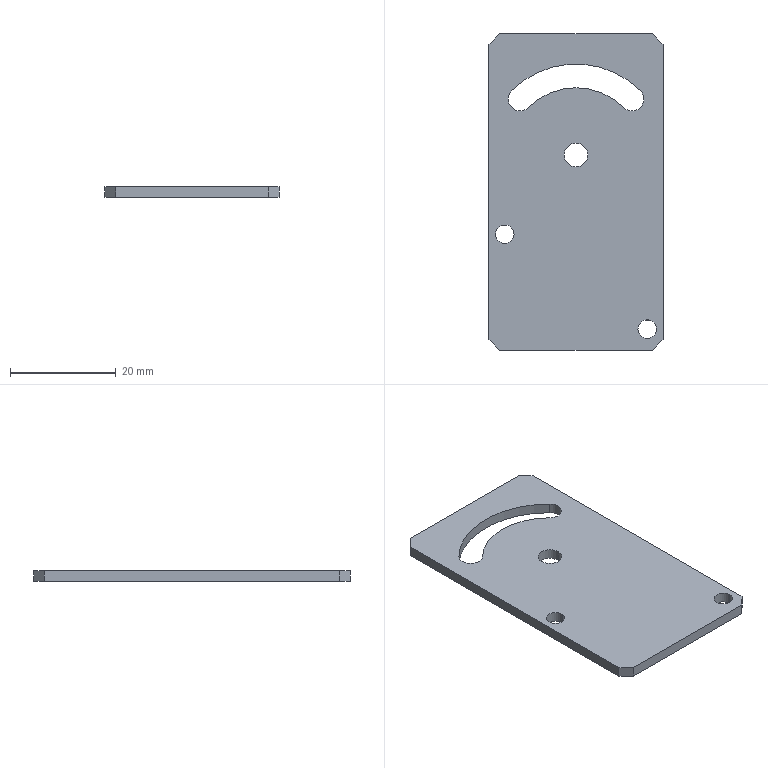Part | SolidWorks | features Chamfer 1, Extrusion 1 | 1 solid | 21 faces | box 33 x 60 x 2 mm | volume 3630 mm3 | cylinder 11 | plane 10 | commonest cylinder face diameters 4.5 x5 3.5 x4 25.5 x1 34.5 x1
STEP:
#1=CARTESIAN_POINT('',(-12.198,19.198,2.));
#2=VERTEX_POINT('',#1);
#3=CARTESIAN_POINT('',(-12.857,17.607,2.));
#4=VERTEX_POINT('',#3);
#5=CARTESIAN_POINT('',(-10.607,17.607,2.));
#6=DIRECTION('',(0.,0.,1.));
#7=DIRECTION('',(1.,0.,0.));
#8=AXIS2_PLACEMENT_3D('',#5,#6,#7);
#9=CIRCLE('',#8,2.25);
#10=EDGE_CURVE('',#2,#4,#9,.T.);
#11=ORIENTED_EDGE('',*,*,#10,.T.);
#12=CARTESIAN_POINT('',(-12.857,17.607,0.));
#13=VERTEX_POINT('',#12);
#14=CARTESIAN_POINT('',(-12.857,17.607,2.));
#15=DIRECTION('',(0.,0.,-1.));
#16=VECTOR('',#15,1000.);
#17=LINE('',#14,#16);
#18=EDGE_CURVE('',#4,#13,#17,.T.);
#19=ORIENTED_EDGE('',*,*,#18,.T.);
#20=CARTESIAN_POINT('',(-12.198,19.198,0.));
#21=VERTEX_POINT('',#20);
#22=CARTESIAN_POINT('',(-10.607,17.607,0.));
#23=DIRECTION('',(0.,0.,1.));
#24=DIRECTION('',(1.,0.,0.));
#25=AXIS2_PLACEMENT_3D('',#22,#23,#24);
#26=CIRCLE('',#25,2.25);
#27=EDGE_CURVE('',#21,#13,#26,.T.);
#28=ORIENTED_EDGE('',*,*,#27,.F.);
#29=CARTESIAN_POINT('',(-12.198,19.198,2.));
#30=DIRECTION('',(0.,0.,-1.));
#31=VECTOR('',#30,1000.);
#32=LINE('',#29,#31);
#33=EDGE_CURVE('',#2,#21,#32,.T.);
#34=ORIENTED_EDGE('',*,*,#33,.F.);
#35=EDGE_LOOP('',(#11,#19,#28,#34));
#36=FACE_OUTER_BOUND('',#35,.T.);
#37=CARTESIAN_POINT('',(-10.607,17.607,2.));
#38=DIRECTION('',(0.,0.,-1.));
#39=DIRECTION('',(-1.,0.,0.));
#40=AXIS2_PLACEMENT_3D('',#37,#38,#39);
#41=CYLINDRICAL_SURFACE('',#40,2.25);
#42=ADVANCED_FACE('',(#36),#41,.F.);
#43=CARTESIAN_POINT('',(-15.25,-8.,2.));
#44=VERTEX_POINT('',#43);
#45=CARTESIAN_POINT('',(-11.75,-8.,2.));
#46=VERTEX_POINT('',#45);
#47=CARTESIAN_POINT('',(-13.5,-8.,2.));
#48=DIRECTION('',(0.,0.,1.));
#49=DIRECTION('',(1.,0.,0.));
#50=AXIS2_PLACEMENT_3D('',#47,#48,#49);
#51=CIRCLE('',#50,1.75);
#52=EDGE_CURVE('',#44,#46,#51,.T.);
#53=ORIENTED_EDGE('',*,*,#52,.T.);
#54=CARTESIAN_POINT('',(-11.75,-8.,0.));
#55=VERTEX_POINT('',#54);
#56=CARTESIAN_POINT('',(-11.75,-8.,2.));
#57=DIRECTION('',(0.,0.,-1.));
#58=VECTOR('',#57,1000.);
#59=LINE('',#56,#58);
#60=EDGE_CURVE('',#46,#55,#59,.T.);
#61=ORIENTED_EDGE('',*,*,#60,.T.);
#62=CARTESIAN_POINT('',(-15.25,-8.,0.));
#63=VERTEX_POINT('',#62);
#64=CARTESIAN_POINT('',(-13.5,-8.,0.));
#65=DIRECTION('',(0.,0.,1.));
#66=DIRECTION('',(1.,0.,0.));
#67=AXIS2_PLACEMENT_3D('',#64,#65,#66);
#68=CIRCLE('',#67,1.75);
#69=EDGE_CURVE('',#63,#55,#68,.T.);
#70=ORIENTED_EDGE('',*,*,#69,.F.);
#71=CARTESIAN_POINT('',(-15.25,-8.,2.));
#72=DIRECTION('',(0.,0.,-1.));
#73=VECTOR('',#72,1000.);
#74=LINE('',#71,#73);
#75=EDGE_CURVE('',#44,#63,#74,.T.);
#76=ORIENTED_EDGE('',*,*,#75,.F.);
#77=EDGE_LOOP('',(#53,#61,#70,#76));
#78=FACE_OUTER_BOUND('',#77,.T.);
#79=CARTESIAN_POINT('',(-13.5,-8.,2.));
#80=DIRECTION('',(0.,0.,-1.));
#81=DIRECTION('',(-1.,0.,0.));
#82=AXIS2_PLACEMENT_3D('',#79,#80,#81);
#83=CYLINDRICAL_SURFACE('',#82,1.75);
#84=ADVANCED_FACE('',(#78),#83,.F.);
#85=CARTESIAN_POINT('',(11.75,-26.,2.));
#86=VERTEX_POINT('',#85);
#87=CARTESIAN_POINT('',(15.25,-26.,2.));
#88=VERTEX_POINT('',#87);
#89=CARTESIAN_POINT('',(13.5,-26.,2.));
#90=DIRECTION('',(0.,0.,1.));
#91=DIRECTION('',(1.,0.,0.));
#92=AXIS2_PLACEMENT_3D('',#89,#90,#91);
#93=CIRCLE('',#92,1.75);
#94=EDGE_CURVE('',#86,#88,#93,.T.);
#95=ORIENTED_EDGE('',*,*,#94,.T.);
#96=CARTESIAN_POINT('',(15.25,-26.,0.));
#97=VERTEX_POINT('',#96);
#98=CARTESIAN_POINT('',(15.25,-26.,2.));
#99=DIRECTION('',(0.,0.,-1.));
#100=VECTOR('',#99,1000.);
#101=LINE('',#98,#100);
#102=EDGE_CURVE('',#88,#97,#101,.T.);
#103=ORIENTED_EDGE('',*,*,#102,.T.);
#104=CARTESIAN_POINT('',(11.75,-26.,0.));
#105=VERTEX_POINT('',#104);
#106=CARTESIAN_POINT('',(13.5,-26.,0.));
#107=DIRECTION('',(0.,0.,1.));
#108=DIRECTION('',(1.,0.,0.));
#109=AXIS2_PLACEMENT_3D('',#106,#107,#108);
#110=CIRCLE('',#109,1.75);
#111=EDGE_CURVE('',#105,#97,#110,.T.);
#112=ORIENTED_EDGE('',*,*,#111,.F.);
#113=CARTESIAN_POINT('',(11.75,-26.,2.));
#114=DIRECTION('',(0.,0.,-1.));
#115=VECTOR('',#114,1000.);
#116=LINE('',#113,#115);
#117=EDGE_CURVE('',#86,#105,#116,.T.);
#118=ORIENTED_EDGE('',*,*,#117,.F.);
#119=EDGE_LOOP('',(#95,#103,#112,#118));
#120=FACE_OUTER_BOUND('',#119,.T.);
#121=CARTESIAN_POINT('',(13.5,-26.,2.));
#122=DIRECTION('',(0.,0.,-1.));
#123=DIRECTION('',(-1.,0.,0.));
#124=AXIS2_PLACEMENT_3D('',#121,#122,#123);
#125=CYLINDRICAL_SURFACE('',#124,1.75);
#126=ADVANCED_FACE('',(#120),#125,.F.);
#127=CARTESIAN_POINT('',(-2.25,7.,2.));
#128=VERTEX_POINT('',#127);
#129=CARTESIAN_POINT('',(2.25,7.,2.));
#130=VERTEX_POINT('',#129);
#131=CARTESIAN_POINT('',(0.,7.,2.));
#132=DIRECTION('',(0.,0.,1.));
#133=DIRECTION('',(1.,0.,0.));
#134=AXIS2_PLACEMENT_3D('',#131,#132,#133);
#135=CIRCLE('',#134,2.25);
#136=EDGE_CURVE('',#128,#130,#135,.T.);
#137=ORIENTED_EDGE('',*,*,#136,.T.);
#138=CARTESIAN_POINT('',(2.25,7.,0.));
#139=VERTEX_POINT('',#138);
#140=CARTESIAN_POINT('',(2.25,7.,2.));
#141=DIRECTION('',(0.,0.,-1.));
#142=VECTOR('',#141,1000.);
#143=LINE('',#140,#142);
#144=EDGE_CURVE('',#130,#139,#143,.T.);
#145=ORIENTED_EDGE('',*,*,#144,.T.);
#146=CARTESIAN_POINT('',(-2.25,7.,0.));
#147=VERTEX_POINT('',#146);
#148=CARTESIAN_POINT('',(0.,7.,0.));
#149=DIRECTION('',(0.,0.,1.));
#150=DIRECTION('',(1.,0.,0.));
#151=AXIS2_PLACEMENT_3D('',#148,#149,#150);
#152=CIRCLE('',#151,2.25);
#153=EDGE_CURVE('',#147,#139,#152,.T.);
#154=ORIENTED_EDGE('',*,*,#153,.F.);
#155=CARTESIAN_POINT('',(-2.25,7.,2.));
#156=DIRECTION('',(0.,0.,-1.));
#157=VECTOR('',#156,1000.);
#158=LINE('',#155,#157);
#159=EDGE_CURVE('',#128,#147,#158,.T.);
#160=ORIENTED_EDGE('',*,*,#159,.F.);
#161=EDGE_LOOP('',(#137,#145,#154,#160));
#162=FACE_OUTER_BOUND('',#161,.T.);
#163=CARTESIAN_POINT('',(0.,7.,2.));
#164=DIRECTION('',(0.,0.,-1.));
#165=DIRECTION('',(-1.,0.,0.));
#166=AXIS2_PLACEMENT_3D('',#163,#164,#165);
#167=CYLINDRICAL_SURFACE('',#166,2.25);
#168=ADVANCED_FACE('',(#162),#167,.F.);
#169=ORIENTED_EDGE('',*,*,#52,.F.);
#170=CARTESIAN_POINT('',(-13.5,-8.,2.));
#171=DIRECTION('',(0.,0.,1.));
#172=DIRECTION('',(1.,0.,0.));
#173=AXIS2_PLACEMENT_3D('',#170,#171,#172);
#174=CIRCLE('',#173,1.75);
#175=EDGE_CURVE('',#46,#44,#174,.T.);
#176=ORIENTED_EDGE('',*,*,#175,.F.);
#177=EDGE_LOOP('',(#169,#176));
#178=FACE_BOUND('',#177,.T.);
#179=ORIENTED_EDGE('',*,*,#94,.F.);
#180=CARTESIAN_POINT('',(13.5,-26.,2.));
#181=DIRECTION('',(0.,0.,1.));
#182=DIRECTION('',(1.,0.,0.));
#183=AXIS2_PLACEMENT_3D('',#180,#181,#182);
#184=CIRCLE('',#183,1.75);
#185=EDGE_CURVE('',#88,#86,#184,.T.);
#186=ORIENTED_EDGE('',*,*,#185,.F.);
#187=EDGE_LOOP('',(#179,#186));
#188=FACE_BOUND('',#187,.T.);
#189=ORIENTED_EDGE('',*,*,#136,.F.);
#190=CARTESIAN_POINT('',(0.,7.,2.));
#191=DIRECTION('',(0.,0.,1.));
#192=DIRECTION('',(1.,0.,0.));
#193=AXIS2_PLACEMENT_3D('',#190,#191,#192);
#194=CIRCLE('',#193,2.25);
#195=EDGE_CURVE('',#130,#128,#194,.T.);
#196=ORIENTED_EDGE('',*,*,#195,.F.);
#197=EDGE_LOOP('',(#189,#196));
#198=FACE_BOUND('',#197,.T.);
#199=CARTESIAN_POINT('',(-14.5,-30.,2.));
#200=VERTEX_POINT('',#199);
#201=CARTESIAN_POINT('',(14.5,-30.,2.));
#202=VERTEX_POINT('',#201);
#203=CARTESIAN_POINT('',(-16.5,-30.,2.));
#204=DIRECTION('',(1.,0.,0.));
#205=VECTOR('',#204,1000.);
#206=LINE('',#203,#205);
#207=EDGE_CURVE('',#200,#202,#206,.T.);
#208=ORIENTED_EDGE('',*,*,#207,.T.);
#209=CARTESIAN_POINT('',(16.5,-28.,2.));
#210=VERTEX_POINT('',#209);
#211=CARTESIAN_POINT('',(16.5,-28.,2.));
#212=DIRECTION('',(0.7071,0.7071,0.));
#213=VECTOR('',#212,1000.);
#214=LINE('',#211,#213);
#215=EDGE_CURVE('',#202,#210,#214,.T.);
#216=ORIENTED_EDGE('',*,*,#215,.T.);
#217=CARTESIAN_POINT('',(16.5,28.,2.));
#218=VERTEX_POINT('',#217);
#219=CARTESIAN_POINT('',(16.5,-30.,2.));
#220=DIRECTION('',(0.,1.,0.));
#221=VECTOR('',#220,1000.);
#222=LINE('',#219,#221);
#223=EDGE_CURVE('',#210,#218,#222,.T.);
#224=ORIENTED_EDGE('',*,*,#223,.T.);
#225=CARTESIAN_POINT('',(14.5,30.,2.));
#226=VERTEX_POINT('',#225);
#227=CARTESIAN_POINT('',(14.5,30.,2.));
#228=DIRECTION('',(-0.7071,0.7071,0.));
#229=VECTOR('',#228,1000.);
#230=LINE('',#227,#229);
#231=EDGE_CURVE('',#218,#226,#230,.T.);
#232=ORIENTED_EDGE('',*,*,#231,.T.);
#233=CARTESIAN_POINT('',(-14.5,30.,2.));
#234=VERTEX_POINT('',#233);
#235=CARTESIAN_POINT('',(-16.5,30.,2.));
#236=DIRECTION('',(-1.,0.,0.));
#237=VECTOR('',#236,1000.);
#238=LINE('',#235,#237);
#239=EDGE_CURVE('',#226,#234,#238,.T.);
#240=ORIENTED_EDGE('',*,*,#239,.T.);
#241=CARTESIAN_POINT('',(-16.5,28.,2.));
#242=VERTEX_POINT('',#241);
#243=CARTESIAN_POINT('',(-16.5,28.,2.));
#244=DIRECTION('',(-0.7071,-0.7071,0.));
#245=VECTOR('',#244,1000.);
#246=LINE('',#243,#245);
#247=EDGE_CURVE('',#234,#242,#246,.T.);
#248=ORIENTED_EDGE('',*,*,#247,.T.);
#249=CARTESIAN_POINT('',(-16.5,-28.,2.));
#250=VERTEX_POINT('',#249);
#251=CARTESIAN_POINT('',(-16.5,-30.,2.));
#252=DIRECTION('',(0.,-1.,0.));
#253=VECTOR('',#252,1000.);
#254=LINE('',#251,#253);
#255=EDGE_CURVE('',#242,#250,#254,.T.);
#256=ORIENTED_EDGE('',*,*,#255,.T.);
#257=CARTESIAN_POINT('',(-14.5,-30.,2.));
#258=DIRECTION('',(0.7071,-0.7071,0.));
#259=VECTOR('',#258,1000.);
#260=LINE('',#257,#259);
#261=EDGE_CURVE('',#250,#200,#260,.T.);
#262=ORIENTED_EDGE('',*,*,#261,.T.);
#263=EDGE_LOOP('',(#208,#216,#224,#232,#240,#248,#256,#262));
#264=FACE_OUTER_BOUND('',#263,.T.);
#265=ORIENTED_EDGE('',*,*,#10,.F.);
#266=CARTESIAN_POINT('',(12.198,19.198,2.));
#267=VERTEX_POINT('',#266);
#268=CARTESIAN_POINT('',(0.,7.,2.));
#269=DIRECTION('',(0.,0.,1.));
#270=DIRECTION('',(1.,0.,0.));
#271=AXIS2_PLACEMENT_3D('',#268,#269,#270);
#272=CIRCLE('',#271,17.25);
#273=EDGE_CURVE('',#267,#2,#272,.T.);
#274=ORIENTED_EDGE('',*,*,#273,.F.);
#275=CARTESIAN_POINT('',(9.016,16.016,2.));
#276=VERTEX_POINT('',#275);
#277=CARTESIAN_POINT('',(10.607,17.607,2.));
#278=DIRECTION('',(0.,0.,1.));
#279=DIRECTION('',(1.,0.,0.));
#280=AXIS2_PLACEMENT_3D('',#277,#278,#279);
#281=CIRCLE('',#280,2.25);
#282=EDGE_CURVE('',#276,#267,#281,.T.);
#283=ORIENTED_EDGE('',*,*,#282,.F.);
#284=CARTESIAN_POINT('',(-9.016,16.016,2.));
#285=VERTEX_POINT('',#284);
#286=CARTESIAN_POINT('',(0.,7.,2.));
#287=DIRECTION('',(0.,0.,-1.));
#288=DIRECTION('',(1.,0.,0.));
#289=AXIS2_PLACEMENT_3D('',#286,#287,#288);
#290=CIRCLE('',#289,12.75);
#291=EDGE_CURVE('',#285,#276,#290,.T.);
#292=ORIENTED_EDGE('',*,*,#291,.F.);
#293=CARTESIAN_POINT('',(-10.607,17.607,2.));
#294=DIRECTION('',(0.,0.,1.));
#295=DIRECTION('',(1.,0.,0.));
#296=AXIS2_PLACEMENT_3D('',#293,#294,#295);
#297=CIRCLE('',#296,2.25);
#298=EDGE_CURVE('',#4,#285,#297,.T.);
#299=ORIENTED_EDGE('',*,*,#298,.F.);
#300=EDGE_LOOP('',(#265,#274,#283,#292,#299));
#301=FACE_BOUND('',#300,.T.);
#302=CARTESIAN_POINT('',(0.,0.,2.));
#303=DIRECTION('',(0.,0.,-1.));
#304=DIRECTION('',(-1.,0.,0.));
#305=AXIS2_PLACEMENT_3D('',#302,#303,#304);
#306=PLANE('',#305);
#307=ADVANCED_FACE('',(#178,#188,#198,#264,#301),#306,.F.);
#308=ORIENTED_EDGE('',*,*,#111,.T.);
#309=CARTESIAN_POINT('',(13.5,-26.,0.));
#310=DIRECTION('',(0.,0.,1.));
#311=DIRECTION('',(1.,0.,0.));
#312=AXIS2_PLACEMENT_3D('',#309,#310,#311);
#313=CIRCLE('',#312,1.75);
#314=EDGE_CURVE('',#97,#105,#313,.T.);
#315=ORIENTED_EDGE('',*,*,#314,.T.);
#316=EDGE_LOOP('',(#308,#315));
#317=FACE_BOUND('',#316,.T.);
#318=CARTESIAN_POINT('',(16.5,-28.,0.));
#319=VERTEX_POINT('',#318);
#320=CARTESIAN_POINT('',(16.5,28.,0.));
#321=VERTEX_POINT('',#320);
#322=CARTESIAN_POINT('',(16.5,-30.,0.));
#323=DIRECTION('',(0.,1.,0.));
#324=VECTOR('',#323,1000.);
#325=LINE('',#322,#324);
#326=EDGE_CURVE('',#319,#321,#325,.T.);
#327=ORIENTED_EDGE('',*,*,#326,.F.);
#328=CARTESIAN_POINT('',(14.5,-30.,0.));
#329=VERTEX_POINT('',#328);
#330=CARTESIAN_POINT('',(22.25,-22.25,0.));
#331=DIRECTION('',(-0.7071,-0.7071,0.));
#332=VECTOR('',#331,1000.);
#333=LINE('',#330,#332);
#334=EDGE_CURVE('',#319,#329,#333,.T.);
#335=ORIENTED_EDGE('',*,*,#334,.T.);
#336=CARTESIAN_POINT('',(-14.5,-30.,0.));
#337=VERTEX_POINT('',#336);
#338=CARTESIAN_POINT('',(-16.5,-30.,0.));
#339=DIRECTION('',(1.,0.,0.));
#340=VECTOR('',#339,1000.);
#341=LINE('',#338,#340);
#342=EDGE_CURVE('',#337,#329,#341,.T.);
#343=ORIENTED_EDGE('',*,*,#342,.F.);
#344=CARTESIAN_POINT('',(-16.5,-28.,0.));
#345=VERTEX_POINT('',#344);
#346=CARTESIAN_POINT('',(-22.25,-22.25,0.));
#347=DIRECTION('',(-0.7071,0.7071,0.));
#348=VECTOR('',#347,1000.);
#349=LINE('',#346,#348);
#350=EDGE_CURVE('',#337,#345,#349,.T.);
#351=ORIENTED_EDGE('',*,*,#350,.T.);
#352=CARTESIAN_POINT('',(-16.5,28.,0.));
#353=VERTEX_POINT('',#352);
#354=CARTESIAN_POINT('',(-16.5,-30.,0.));
#355=DIRECTION('',(0.,-1.,0.));
#356=VECTOR('',#355,1000.);
#357=LINE('',#354,#356);
#358=EDGE_CURVE('',#353,#345,#357,.T.);
#359=ORIENTED_EDGE('',*,*,#358,.F.);
#360=CARTESIAN_POINT('',(-14.5,30.,0.));
#361=VERTEX_POINT('',#360);
#362=CARTESIAN_POINT('',(-22.25,22.25,0.));
#363=DIRECTION('',(0.7071,0.7071,0.));
#364=VECTOR('',#363,1000.);
#365=LINE('',#362,#364);
#366=EDGE_CURVE('',#353,#361,#365,.T.);
#367=ORIENTED_EDGE('',*,*,#366,.T.);
#368=CARTESIAN_POINT('',(14.5,30.,0.));
#369=VERTEX_POINT('',#368);
#370=CARTESIAN_POINT('',(-16.5,30.,0.));
#371=DIRECTION('',(-1.,0.,0.));
#372=VECTOR('',#371,1000.);
#373=LINE('',#370,#372);
#374=EDGE_CURVE('',#369,#361,#373,.T.);
#375=ORIENTED_EDGE('',*,*,#374,.F.);
#376=CARTESIAN_POINT('',(22.25,22.25,0.));
#377=DIRECTION('',(0.7071,-0.7071,0.));
#378=VECTOR('',#377,1000.);
#379=LINE('',#376,#378);
#380=EDGE_CURVE('',#369,#321,#379,.T.);
#381=ORIENTED_EDGE('',*,*,#380,.T.);
#382=EDGE_LOOP('',(#327,#335,#343,#351,#359,#367,#375,#381));
#383=FACE_OUTER_BOUND('',#382,.T.);
#384=ORIENTED_EDGE('',*,*,#153,.T.);
#385=CARTESIAN_POINT('',(0.,7.,0.));
#386=DIRECTION('',(0.,0.,1.));
#387=DIRECTION('',(1.,0.,0.));
#388=AXIS2_PLACEMENT_3D('',#385,#386,#387);
#389=CIRCLE('',#388,2.25);
#390=EDGE_CURVE('',#139,#147,#389,.T.);
#391=ORIENTED_EDGE('',*,*,#390,.T.);
#392=EDGE_LOOP('',(#384,#391));
#393=FACE_BOUND('',#392,.T.);
#394=ORIENTED_EDGE('',*,*,#69,.T.);
#395=CARTESIAN_POINT('',(-13.5,-8.,0.));
#396=DIRECTION('',(0.,0.,1.));
#397=DIRECTION('',(1.,0.,0.));
#398=AXIS2_PLACEMENT_3D('',#395,#396,#397);
#399=CIRCLE('',#398,1.75);
#400=EDGE_CURVE('',#55,#63,#399,.T.);
#401=ORIENTED_EDGE('',*,*,#400,.T.);
#402=EDGE_LOOP('',(#394,#401));
#403=FACE_BOUND('',#402,.T.);
#404=CARTESIAN_POINT('',(12.198,19.198,0.));
#405=VERTEX_POINT('',#404);
#406=CARTESIAN_POINT('',(0.,7.,0.));
#407=DIRECTION('',(0.,0.,1.));
#408=DIRECTION('',(1.,0.,0.));
#409=AXIS2_PLACEMENT_3D('',#406,#407,#408);
#410=CIRCLE('',#409,17.25);
#411=EDGE_CURVE('',#405,#21,#410,.T.);
#412=ORIENTED_EDGE('',*,*,#411,.T.);
#413=ORIENTED_EDGE('',*,*,#27,.T.);
#414=CARTESIAN_POINT('',(-9.016,16.016,0.));
#415=VERTEX_POINT('',#414);
#416=CARTESIAN_POINT('',(-10.607,17.607,0.));
#417=DIRECTION('',(0.,0.,1.));
#418=DIRECTION('',(1.,0.,0.));
#419=AXIS2_PLACEMENT_3D('',#416,#417,#418);
#420=CIRCLE('',#419,2.25);
#421=EDGE_CURVE('',#13,#415,#420,.T.);
#422=ORIENTED_EDGE('',*,*,#421,.T.);
#423=CARTESIAN_POINT('',(9.016,16.016,0.));
#424=VERTEX_POINT('',#423);
#425=CARTESIAN_POINT('',(0.,7.,0.));
#426=DIRECTION('',(0.,0.,-1.));
#427=DIRECTION('',(1.,0.,0.));
#428=AXIS2_PLACEMENT_3D('',#425,#426,#427);
#429=CIRCLE('',#428,12.75);
#430=EDGE_CURVE('',#415,#424,#429,.T.);
#431=ORIENTED_EDGE('',*,*,#430,.T.);
#432=CARTESIAN_POINT('',(10.607,17.607,0.));
#433=DIRECTION('',(0.,0.,1.));
#434=DIRECTION('',(1.,0.,0.));
#435=AXIS2_PLACEMENT_3D('',#432,#433,#434);
#436=CIRCLE('',#435,2.25);
#437=EDGE_CURVE('',#424,#405,#436,.T.);
#438=ORIENTED_EDGE('',*,*,#437,.T.);
#439=EDGE_LOOP('',(#412,#413,#422,#431,#438));
#440=FACE_BOUND('',#439,.T.);
#441=CARTESIAN_POINT('',(0.,0.,0.));
#442=DIRECTION('',(0.,0.,-1.));
#443=DIRECTION('',(-1.,0.,0.));
#444=AXIS2_PLACEMENT_3D('',#441,#442,#443);
#445=PLANE('',#444);
#446=ADVANCED_FACE('',(#317,#383,#393,#403,#440),#445,.T.);
#447=ORIENTED_EDGE('',*,*,#223,.F.);
#448=CARTESIAN_POINT('',(16.5,-28.,2.));
#449=DIRECTION('',(0.,0.,-1.));
#450=VECTOR('',#449,1000.);
#451=LINE('',#448,#450);
#452=EDGE_CURVE('',#210,#319,#451,.T.);
#453=ORIENTED_EDGE('',*,*,#452,.T.);
#454=ORIENTED_EDGE('',*,*,#326,.T.);
#455=CARTESIAN_POINT('',(16.5,28.,2.));
#456=DIRECTION('',(0.,0.,1.));
#457=VECTOR('',#456,1000.);
#458=LINE('',#455,#457);
#459=EDGE_CURVE('',#321,#218,#458,.T.);
#460=ORIENTED_EDGE('',*,*,#459,.T.);
#461=EDGE_LOOP('',(#447,#453,#454,#460));
#462=FACE_OUTER_BOUND('',#461,.T.);
#463=CARTESIAN_POINT('',(16.5,-30.,2.));
#464=DIRECTION('',(-1.,0.,0.));
#465=DIRECTION('',(0.,0.,1.));
#466=AXIS2_PLACEMENT_3D('',#463,#464,#465);
#467=PLANE('',#466);
#468=ADVANCED_FACE('',(#462),#467,.F.);
#469=ORIENTED_EDGE('',*,*,#239,.F.);
#470=CARTESIAN_POINT('',(14.5,30.,2.));
#471=DIRECTION('',(0.,0.,-1.));
#472=VECTOR('',#471,1000.);
#473=LINE('',#470,#472);
#474=EDGE_CURVE('',#226,#369,#473,.T.);
#475=ORIENTED_EDGE('',*,*,#474,.T.);
#476=ORIENTED_EDGE('',*,*,#374,.T.);
#477=CARTESIAN_POINT('',(-14.5,30.,2.));
#478=DIRECTION('',(0.,0.,1.));
#479=VECTOR('',#478,1000.);
#480=LINE('',#477,#479);
#481=EDGE_CURVE('',#361,#234,#480,.T.);
#482=ORIENTED_EDGE('',*,*,#481,.T.);
#483=EDGE_LOOP('',(#469,#475,#476,#482));
#484=FACE_OUTER_BOUND('',#483,.T.);
#485=CARTESIAN_POINT('',(-16.5,30.,2.));
#486=DIRECTION('',(0.,-1.,0.));
#487=DIRECTION('',(0.,0.,-1.));
#488=AXIS2_PLACEMENT_3D('',#485,#486,#487);
#489=PLANE('',#488);
#490=ADVANCED_FACE('',(#484),#489,.F.);
#491=ORIENTED_EDGE('',*,*,#358,.T.);
#492=CARTESIAN_POINT('',(-16.5,-28.,2.));
#493=DIRECTION('',(0.,0.,1.));
#494=VECTOR('',#493,1000.);
#495=LINE('',#492,#494);
#496=EDGE_CURVE('',#345,#250,#495,.T.);
#497=ORIENTED_EDGE('',*,*,#496,.T.);
#498=ORIENTED_EDGE('',*,*,#255,.F.);
#499=CARTESIAN_POINT('',(-16.5,28.,2.));
#500=DIRECTION('',(0.,0.,-1.));
#501=VECTOR('',#500,1000.);
#502=LINE('',#499,#501);
#503=EDGE_CURVE('',#242,#353,#502,.T.);
#504=ORIENTED_EDGE('',*,*,#503,.T.);
#505=EDGE_LOOP('',(#491,#497,#498,#504));
#506=FACE_OUTER_BOUND('',#505,.T.);
#507=CARTESIAN_POINT('',(-16.5,-30.,2.));
#508=DIRECTION('',(1.,0.,0.));
#509=DIRECTION('',(0.,0.,-1.));
#510=AXIS2_PLACEMENT_3D('',#507,#508,#509);
#511=PLANE('',#510);
#512=ADVANCED_FACE('',(#506),#511,.F.);
#513=ORIENTED_EDGE('',*,*,#342,.T.);
#514=CARTESIAN_POINT('',(14.5,-30.,2.));
#515=DIRECTION('',(0.,0.,1.));
#516=VECTOR('',#515,1000.);
#517=LINE('',#514,#516);
#518=EDGE_CURVE('',#329,#202,#517,.T.);
#519=ORIENTED_EDGE('',*,*,#518,.T.);
#520=ORIENTED_EDGE('',*,*,#207,.F.);
#521=CARTESIAN_POINT('',(-14.5,-30.,2.));
#522=DIRECTION('',(0.,0.,-1.));
#523=VECTOR('',#522,1000.);
#524=LINE('',#521,#523);
#525=EDGE_CURVE('',#200,#337,#524,.T.);
#526=ORIENTED_EDGE('',*,*,#525,.T.);
#527=EDGE_LOOP('',(#513,#519,#520,#526));
#528=FACE_OUTER_BOUND('',#527,.T.);
#529=CARTESIAN_POINT('',(-16.5,-30.,2.));
#530=DIRECTION('',(0.,1.,0.));
#531=DIRECTION('',(0.,0.,1.));
#532=AXIS2_PLACEMENT_3D('',#529,#530,#531);
#533=PLANE('',#532);
#534=ADVANCED_FACE('',(#528),#533,.F.);
#535=ORIENTED_EDGE('',*,*,#144,.F.);
#536=ORIENTED_EDGE('',*,*,#195,.T.);
#537=ORIENTED_EDGE('',*,*,#159,.T.);
#538=ORIENTED_EDGE('',*,*,#390,.F.);
#539=EDGE_LOOP('',(#535,#536,#537,#538));
#540=FACE_OUTER_BOUND('',#539,.T.);
#541=CARTESIAN_POINT('',(0.,7.,2.));
#542=DIRECTION('',(0.,0.,-1.));
#543=DIRECTION('',(-1.,0.,0.));
#544=AXIS2_PLACEMENT_3D('',#541,#542,#543);
#545=CYLINDRICAL_SURFACE('',#544,2.25);
#546=ADVANCED_FACE('',(#540),#545,.F.);
#547=ORIENTED_EDGE('',*,*,#102,.F.);
#548=ORIENTED_EDGE('',*,*,#185,.T.);
#549=ORIENTED_EDGE('',*,*,#117,.T.);
#550=ORIENTED_EDGE('',*,*,#314,.F.);
#551=EDGE_LOOP('',(#547,#548,#549,#550));
#552=FACE_OUTER_BOUND('',#551,.T.);
#553=CARTESIAN_POINT('',(13.5,-26.,2.));
#554=DIRECTION('',(0.,0.,-1.));
#555=DIRECTION('',(-1.,0.,0.));
#556=AXIS2_PLACEMENT_3D('',#553,#554,#555);
#557=CYLINDRICAL_SURFACE('',#556,1.75);
#558=ADVANCED_FACE('',(#552),#557,.F.);
#559=ORIENTED_EDGE('',*,*,#60,.F.);
#560=ORIENTED_EDGE('',*,*,#175,.T.);
#561=ORIENTED_EDGE('',*,*,#75,.T.);
#562=ORIENTED_EDGE('',*,*,#400,.F.);
#563=EDGE_LOOP('',(#559,#560,#561,#562));
#564=FACE_OUTER_BOUND('',#563,.T.);
#565=CARTESIAN_POINT('',(-13.5,-8.,2.));
#566=DIRECTION('',(0.,0.,-1.));
#567=DIRECTION('',(-1.,0.,0.));
#568=AXIS2_PLACEMENT_3D('',#565,#566,#567);
#569=CYLINDRICAL_SURFACE('',#568,1.75);
#570=ADVANCED_FACE('',(#564),#569,.F.);
#571=ORIENTED_EDGE('',*,*,#18,.F.);
#572=ORIENTED_EDGE('',*,*,#298,.T.);
#573=CARTESIAN_POINT('',(-9.016,16.016,2.));
#574=DIRECTION('',(0.,0.,-1.));
#575=VECTOR('',#574,1000.);
#576=LINE('',#573,#575);
#577=EDGE_CURVE('',#285,#415,#576,.T.);
#578=ORIENTED_EDGE('',*,*,#577,.T.);
#579=ORIENTED_EDGE('',*,*,#421,.F.);
#580=EDGE_LOOP('',(#571,#572,#578,#579));
#581=FACE_OUTER_BOUND('',#580,.T.);
#582=CARTESIAN_POINT('',(-10.607,17.607,2.));
#583=DIRECTION('',(0.,0.,-1.));
#584=DIRECTION('',(-1.,0.,0.));
#585=AXIS2_PLACEMENT_3D('',#582,#583,#584);
#586=CYLINDRICAL_SURFACE('',#585,2.25);
#587=ADVANCED_FACE('',(#581),#586,.F.);
#588=ORIENTED_EDGE('',*,*,#430,.F.);
#589=ORIENTED_EDGE('',*,*,#577,.F.);
#590=ORIENTED_EDGE('',*,*,#291,.T.);
#591=CARTESIAN_POINT('',(9.016,16.016,2.));
#592=DIRECTION('',(0.,0.,-1.));
#593=VECTOR('',#592,1000.);
#594=LINE('',#591,#593);
#595=EDGE_CURVE('',#276,#424,#594,.T.);
#596=ORIENTED_EDGE('',*,*,#595,.T.);
#597=EDGE_LOOP('',(#588,#589,#590,#596));
#598=FACE_OUTER_BOUND('',#597,.T.);
#599=CARTESIAN_POINT('',(0.,7.,2.));
#600=DIRECTION('',(0.,0.,-1.));
#601=DIRECTION('',(-1.,0.,0.));
#602=AXIS2_PLACEMENT_3D('',#599,#600,#601);
#603=CYLINDRICAL_SURFACE('',#602,12.75);
#604=ADVANCED_FACE('',(#598),#603,.T.);
#605=ORIENTED_EDGE('',*,*,#437,.F.);
#606=ORIENTED_EDGE('',*,*,#595,.F.);
#607=ORIENTED_EDGE('',*,*,#282,.T.);
#608=CARTESIAN_POINT('',(12.198,19.198,2.));
#609=DIRECTION('',(0.,0.,-1.));
#610=VECTOR('',#609,1000.);
#611=LINE('',#608,#610);
#612=EDGE_CURVE('',#267,#405,#611,.T.);
#613=ORIENTED_EDGE('',*,*,#612,.T.);
#614=EDGE_LOOP('',(#605,#606,#607,#613));
#615=FACE_OUTER_BOUND('',#614,.T.);
#616=CARTESIAN_POINT('',(10.607,17.607,2.));
#617=DIRECTION('',(0.,0.,-1.));
#618=DIRECTION('',(-1.,0.,0.));
#619=AXIS2_PLACEMENT_3D('',#616,#617,#618);
#620=CYLINDRICAL_SURFACE('',#619,2.25);
#621=ADVANCED_FACE('',(#615),#620,.F.);
#622=ORIENTED_EDGE('',*,*,#411,.F.);
#623=ORIENTED_EDGE('',*,*,#612,.F.);
#624=ORIENTED_EDGE('',*,*,#273,.T.);
#625=ORIENTED_EDGE('',*,*,#33,.T.);
#626=EDGE_LOOP('',(#622,#623,#624,#625));
#627=FACE_OUTER_BOUND('',#626,.T.);
#628=CARTESIAN_POINT('',(0.,7.,2.));
#629=DIRECTION('',(0.,0.,-1.));
#630=DIRECTION('',(-1.,0.,0.));
#631=AXIS2_PLACEMENT_3D('',#628,#629,#630);
#632=CYLINDRICAL_SURFACE('',#631,17.25);
#633=ADVANCED_FACE('',(#627),#632,.F.);
#634=ORIENTED_EDGE('',*,*,#215,.F.);
#635=ORIENTED_EDGE('',*,*,#518,.F.);
#636=ORIENTED_EDGE('',*,*,#334,.F.);
#637=ORIENTED_EDGE('',*,*,#452,.F.);
#638=EDGE_LOOP('',(#634,#635,#636,#637));
#639=FACE_OUTER_BOUND('',#638,.T.);
#640=CARTESIAN_POINT('',(16.5,-28.,2.));
#641=DIRECTION('',(-0.7071,0.7071,0.));
#642=DIRECTION('',(0.,0.,-1.));
#643=AXIS2_PLACEMENT_3D('',#640,#641,#642);
#644=PLANE('',#643);
#645=ADVANCED_FACE('',(#639),#644,.F.);
#646=ORIENTED_EDGE('',*,*,#261,.F.);
#647=ORIENTED_EDGE('',*,*,#496,.F.);
#648=ORIENTED_EDGE('',*,*,#350,.F.);
#649=ORIENTED_EDGE('',*,*,#525,.F.);
#650=EDGE_LOOP('',(#646,#647,#648,#649));
#651=FACE_OUTER_BOUND('',#650,.T.);
#652=CARTESIAN_POINT('',(-14.5,-30.,2.));
#653=DIRECTION('',(0.7071,0.7071,0.));
#654=DIRECTION('',(0.,0.,-1.));
#655=AXIS2_PLACEMENT_3D('',#652,#653,#654);
#656=PLANE('',#655);
#657=ADVANCED_FACE('',(#651),#656,.F.);
#658=ORIENTED_EDGE('',*,*,#231,.F.);
#659=ORIENTED_EDGE('',*,*,#459,.F.);
#660=ORIENTED_EDGE('',*,*,#380,.F.);
#661=ORIENTED_EDGE('',*,*,#474,.F.);
#662=EDGE_LOOP('',(#658,#659,#660,#661));
#663=FACE_OUTER_BOUND('',#662,.T.);
#664=CARTESIAN_POINT('',(14.5,30.,2.));
#665=DIRECTION('',(-0.7071,-0.7071,0.));
#666=DIRECTION('',(0.,0.,-1.));
#667=AXIS2_PLACEMENT_3D('',#664,#665,#666);
#668=PLANE('',#667);
#669=ADVANCED_FACE('',(#663),#668,.F.);
#670=ORIENTED_EDGE('',*,*,#247,.F.);
#671=ORIENTED_EDGE('',*,*,#481,.F.);
#672=ORIENTED_EDGE('',*,*,#366,.F.);
#673=ORIENTED_EDGE('',*,*,#503,.F.);
#674=EDGE_LOOP('',(#670,#671,#672,#673));
#675=FACE_OUTER_BOUND('',#674,.T.);
#676=CARTESIAN_POINT('',(-16.5,28.,2.));
#677=DIRECTION('',(0.7071,-0.7071,0.));
#678=DIRECTION('',(0.,0.,-1.));
#679=AXIS2_PLACEMENT_3D('',#676,#677,#678);
#680=PLANE('',#679);
#681=ADVANCED_FACE('',(#675),#680,.F.);
#682=CLOSED_SHELL('',(#42,#84,#126,#168,#307,#446,#468,#490,#512,#534,#546,#558,#570,#587,#604,#621,#633,#645,#657,#669,#681));
#683=MANIFOLD_SOLID_BREP('',#682);
#684=CARTESIAN_POINT('',(0.,0.,0.));
#685=DIRECTION('',(0.,0.,1.));
#686=DIRECTION('',(1.,0.,0.));
#687=AXIS2_PLACEMENT_3D('',#684,#685,#686);
#688=(LENGTH_UNIT()NAMED_UNIT(*)SI_UNIT(.MILLI.,.METRE.));
#689=UNCERTAINTY_MEASURE_WITH_UNIT(LENGTH_MEASURE(0.00001),#688,'','');
#690=(NAMED_UNIT(*)PLANE_ANGLE_UNIT()SI_UNIT($,.RADIAN.));
#691=(NAMED_UNIT(*)SI_UNIT($,.STERADIAN.)SOLID_ANGLE_UNIT());
#692=(GEOMETRIC_REPRESENTATION_CONTEXT(3)GLOBAL_UNCERTAINTY_ASSIGNED_CONTEXT((#689))GLOBAL_UNIT_ASSIGNED_CONTEXT((#688,#690,#691))REPRESENTATION_CONTEXT('',''));
#693=ADVANCED_BREP_SHAPE_REPRESENTATION('',(#683,#687),#692);